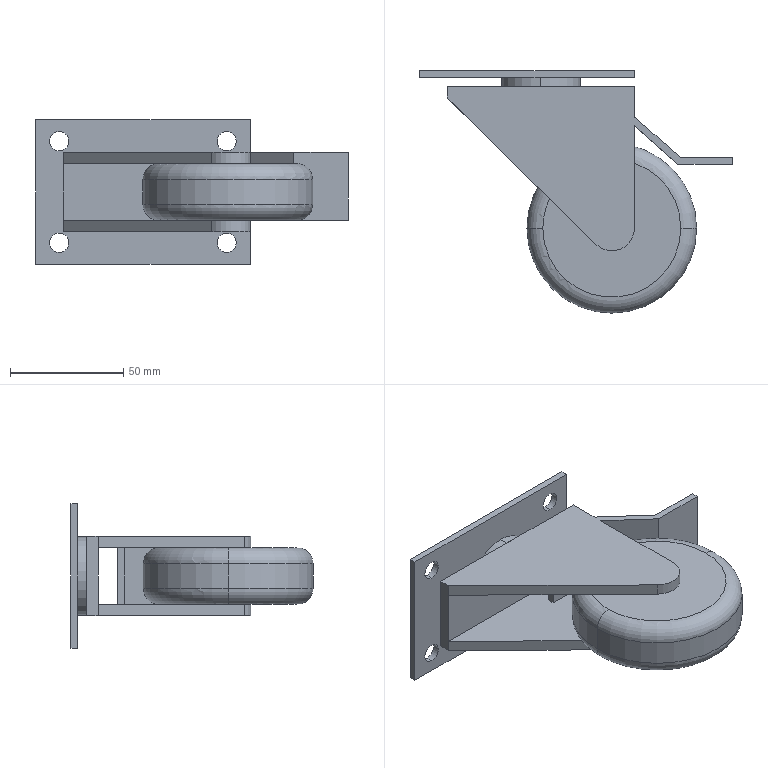Part | SolidWorks | features ICE 7, BossThin 1, Extrusion 1, Fillet 1, MirrorPattern 1 | 1 solid | 47 faces | box 138.347 x 107 x 64 mm | volume 180748 mm3 | plane 29 | cylinder 14 | torus 4 | commonest cylinder face diameters 8.5 x8 20 x2 35 x2 75 x2
STEP:
#1=CARTESIAN_POINT('',(-37.5,0.,5.5));
#2=VERTEX_POINT('',#1);
#3=CARTESIAN_POINT('',(37.5,0.,5.5));
#4=VERTEX_POINT('',#3);
#5=CARTESIAN_POINT('',(0.,0.,5.5));
#6=DIRECTION('',(0.,0.,-1.));
#7=DIRECTION('',(1.,0.,0.));
#8=AXIS2_PLACEMENT_3D('',#5,#6,#7);
#9=CIRCLE('',#8,37.5);
#10=EDGE_CURVE('',#2,#4,#9,.T.);
#11=ORIENTED_EDGE('',*,*,#10,.F.);
#12=CARTESIAN_POINT('',(-30.5,0.,12.5));
#13=VERTEX_POINT('',#12);
#14=CARTESIAN_POINT('',(-30.5,0.,5.5));
#15=DIRECTION('',(0.,1.,0.));
#16=DIRECTION('',(-1.,0.,0.));
#17=AXIS2_PLACEMENT_3D('',#14,#15,#16);
#18=CIRCLE('',#17,7.);
#19=EDGE_CURVE('',#2,#13,#18,.T.);
#20=ORIENTED_EDGE('',*,*,#19,.T.);
#21=CARTESIAN_POINT('',(-27.561,13.062,12.5));
#22=VERTEX_POINT('',#21);
#23=CARTESIAN_POINT('',(0.,0.,12.5));
#24=DIRECTION('',(0.,0.,1.));
#25=DIRECTION('',(1.,0.,0.));
#26=AXIS2_PLACEMENT_3D('',#23,#24,#25);
#27=CIRCLE('',#26,30.5);
#28=EDGE_CURVE('',#22,#13,#27,.T.);
#29=ORIENTED_EDGE('',*,*,#28,.F.);
#30=CARTESIAN_POINT('',(10.,28.814,12.5));
#31=VERTEX_POINT('',#30);
#32=CARTESIAN_POINT('',(0.,0.,12.5));
#33=DIRECTION('',(0.,0.,1.));
#34=DIRECTION('',(1.,0.,0.));
#35=AXIS2_PLACEMENT_3D('',#32,#33,#34);
#36=CIRCLE('',#35,30.5);
#37=EDGE_CURVE('',#31,#22,#36,.T.);
#38=ORIENTED_EDGE('',*,*,#37,.F.);
#39=CARTESIAN_POINT('',(30.5,0.,12.5));
#40=VERTEX_POINT('',#39);
#41=CARTESIAN_POINT('',(0.,0.,12.5));
#42=DIRECTION('',(0.,0.,1.));
#43=DIRECTION('',(1.,0.,0.));
#44=AXIS2_PLACEMENT_3D('',#41,#42,#43);
#45=CIRCLE('',#44,30.5);
#46=EDGE_CURVE('',#40,#31,#45,.T.);
#47=ORIENTED_EDGE('',*,*,#46,.F.);
#48=CARTESIAN_POINT('',(30.5,0.,5.5));
#49=DIRECTION('',(0.,-1.,0.));
#50=DIRECTION('',(0.,0.,-1.));
#51=AXIS2_PLACEMENT_3D('',#48,#49,#50);
#52=CIRCLE('',#51,7.);
#53=EDGE_CURVE('',#4,#40,#52,.T.);
#54=ORIENTED_EDGE('',*,*,#53,.F.);
#55=EDGE_LOOP('',(#11,#20,#29,#38,#47,#54));
#56=FACE_OUTER_BOUND('',#55,.T.);
#57=CARTESIAN_POINT('',(0.,0.,5.5));
#58=DIRECTION('',(0.,0.,1.));
#59=DIRECTION('',(1.,0.,0.));
#60=AXIS2_PLACEMENT_3D('',#57,#58,#59);
#61=TOROIDAL_SURFACE('',#60,30.5,7.);
#62=ADVANCED_FACE('',(#56),#61,.T.);
#63=CARTESIAN_POINT('',(-30.5,0.,-12.5));
#64=VERTEX_POINT('',#63);
#65=CARTESIAN_POINT('',(-27.561,13.062,-12.5));
#66=VERTEX_POINT('',#65);
#67=CARTESIAN_POINT('',(0.,0.,-12.5));
#68=DIRECTION('',(0.,0.,-1.));
#69=DIRECTION('',(1.,0.,0.));
#70=AXIS2_PLACEMENT_3D('',#67,#68,#69);
#71=CIRCLE('',#70,30.5);
#72=EDGE_CURVE('',#64,#66,#71,.T.);
#73=ORIENTED_EDGE('',*,*,#72,.F.);
#74=CARTESIAN_POINT('',(-37.5,0.,-5.5));
#75=VERTEX_POINT('',#74);
#76=CARTESIAN_POINT('',(-30.5,0.,-5.5));
#77=DIRECTION('',(0.,1.,0.));
#78=DIRECTION('',(-1.,0.,0.));
#79=AXIS2_PLACEMENT_3D('',#76,#77,#78);
#80=CIRCLE('',#79,7.);
#81=EDGE_CURVE('',#64,#75,#80,.T.);
#82=ORIENTED_EDGE('',*,*,#81,.T.);
#83=CARTESIAN_POINT('',(37.5,0.,-5.5));
#84=VERTEX_POINT('',#83);
#85=CARTESIAN_POINT('',(0.,0.,-5.5));
#86=DIRECTION('',(0.,0.,1.));
#87=DIRECTION('',(1.,0.,0.));
#88=AXIS2_PLACEMENT_3D('',#85,#86,#87);
#89=CIRCLE('',#88,37.5);
#90=EDGE_CURVE('',#84,#75,#89,.T.);
#91=ORIENTED_EDGE('',*,*,#90,.F.);
#92=CARTESIAN_POINT('',(30.5,0.,-12.5));
#93=VERTEX_POINT('',#92);
#94=CARTESIAN_POINT('',(30.5,0.,-5.5));
#95=DIRECTION('',(0.,-1.,0.));
#96=DIRECTION('',(0.,0.,-1.));
#97=AXIS2_PLACEMENT_3D('',#94,#95,#96);
#98=CIRCLE('',#97,7.);
#99=EDGE_CURVE('',#93,#84,#98,.T.);
#100=ORIENTED_EDGE('',*,*,#99,.F.);
#101=CARTESIAN_POINT('',(10.,28.814,-12.5));
#102=VERTEX_POINT('',#101);
#103=CARTESIAN_POINT('',(0.,0.,-12.5));
#104=DIRECTION('',(0.,0.,-1.));
#105=DIRECTION('',(1.,0.,0.));
#106=AXIS2_PLACEMENT_3D('',#103,#104,#105);
#107=CIRCLE('',#106,30.5);
#108=EDGE_CURVE('',#102,#93,#107,.T.);
#109=ORIENTED_EDGE('',*,*,#108,.F.);
#110=CARTESIAN_POINT('',(0.,0.,-12.5));
#111=DIRECTION('',(0.,0.,-1.));
#112=DIRECTION('',(1.,0.,0.));
#113=AXIS2_PLACEMENT_3D('',#110,#111,#112);
#114=CIRCLE('',#113,30.5);
#115=EDGE_CURVE('',#66,#102,#114,.T.);
#116=ORIENTED_EDGE('',*,*,#115,.F.);
#117=EDGE_LOOP('',(#73,#82,#91,#100,#109,#116));
#118=FACE_OUTER_BOUND('',#117,.T.);
#119=CARTESIAN_POINT('',(0.,0.,-5.5));
#120=DIRECTION('',(0.,0.,1.));
#121=DIRECTION('',(1.,0.,0.));
#122=AXIS2_PLACEMENT_3D('',#119,#120,#121);
#123=TOROIDAL_SURFACE('',#122,30.5,7.);
#124=ADVANCED_FACE('',(#118),#123,.T.);
#125=ORIENTED_EDGE('',*,*,#10,.T.);
#126=CARTESIAN_POINT('',(37.5,0.,12.5));
#127=DIRECTION('',(0.,0.,-1.));
#128=VECTOR('',#127,1000.);
#129=LINE('',#126,#128);
#130=EDGE_CURVE('',#4,#84,#129,.T.);
#131=ORIENTED_EDGE('',*,*,#130,.T.);
#132=ORIENTED_EDGE('',*,*,#90,.T.);
#133=CARTESIAN_POINT('',(-37.5,0.,12.5));
#134=DIRECTION('',(0.,0.,-1.));
#135=VECTOR('',#134,1000.);
#136=LINE('',#133,#135);
#137=EDGE_CURVE('',#2,#75,#136,.T.);
#138=ORIENTED_EDGE('',*,*,#137,.F.);
#139=EDGE_LOOP('',(#125,#131,#132,#138));
#140=FACE_OUTER_BOUND('',#139,.T.);
#141=CARTESIAN_POINT('',(0.,0.,12.5));
#142=DIRECTION('',(0.,0.,-1.));
#143=DIRECTION('',(-1.,0.,0.));
#144=AXIS2_PLACEMENT_3D('',#141,#142,#143);
#145=CYLINDRICAL_SURFACE('',#144,37.5);
#146=ADVANCED_FACE('',(#140),#145,.T.);
#147=CARTESIAN_POINT('',(-31.403,66.5,-17.5));
#148=VERTEX_POINT('',#147);
#149=CARTESIAN_POINT('',(-31.403,66.5,17.5));
#150=VERTEX_POINT('',#149);
#151=CARTESIAN_POINT('',(-31.403,66.5,0.));
#152=DIRECTION('',(0.,-1.,0.));
#153=DIRECTION('',(0.,0.,1.));
#154=AXIS2_PLACEMENT_3D('',#151,#152,#153);
#155=CIRCLE('',#154,17.5);
#156=EDGE_CURVE('',#148,#150,#155,.T.);
#157=ORIENTED_EDGE('',*,*,#156,.T.);
#158=CARTESIAN_POINT('',(-31.403,62.518,17.5));
#159=VERTEX_POINT('',#158);
#160=CARTESIAN_POINT('',(-31.403,115.997,17.5));
#161=DIRECTION('',(0.,-1.,0.));
#162=VECTOR('',#161,1000.);
#163=LINE('',#160,#162);
#164=EDGE_CURVE('',#150,#159,#163,.T.);
#165=ORIENTED_EDGE('',*,*,#164,.T.);
#166=CARTESIAN_POINT('',(-31.403,62.518,-17.5));
#167=VERTEX_POINT('',#166);
#168=CARTESIAN_POINT('',(-31.403,62.518,0.));
#169=DIRECTION('',(0.,1.,0.));
#170=DIRECTION('',(0.,0.,1.));
#171=AXIS2_PLACEMENT_3D('',#168,#169,#170);
#172=CIRCLE('',#171,17.5);
#173=EDGE_CURVE('',#159,#167,#172,.T.);
#174=ORIENTED_EDGE('',*,*,#173,.T.);
#175=CARTESIAN_POINT('',(-31.403,115.997,-17.5));
#176=DIRECTION('',(0.,-1.,0.));
#177=VECTOR('',#176,1000.);
#178=LINE('',#175,#177);
#179=EDGE_CURVE('',#148,#167,#178,.T.);
#180=ORIENTED_EDGE('',*,*,#179,.F.);
#181=EDGE_LOOP('',(#157,#165,#174,#180));
#182=FACE_OUTER_BOUND('',#181,.T.);
#183=CARTESIAN_POINT('',(-31.403,115.997,0.));
#184=DIRECTION('',(0.,-1.,0.));
#185=DIRECTION('',(0.,0.,-1.));
#186=AXIS2_PLACEMENT_3D('',#183,#184,#185);
#187=CYLINDRICAL_SURFACE('',#186,17.5);
#188=ADVANCED_FACE('',(#182),#187,.T.);
#189=CARTESIAN_POINT('',(-74.5,66.5,18.15));
#190=VERTEX_POINT('',#189);
#191=CARTESIAN_POINT('',(-74.5,66.5,26.65));
#192=VERTEX_POINT('',#191);
#193=CARTESIAN_POINT('',(-74.5,66.5,22.4));
#194=DIRECTION('',(0.,1.,0.));
#195=DIRECTION('',(0.,0.,1.));
#196=AXIS2_PLACEMENT_3D('',#193,#194,#195);
#197=CIRCLE('',#196,4.25);
#198=EDGE_CURVE('',#190,#192,#197,.T.);
#199=ORIENTED_EDGE('',*,*,#198,.F.);
#200=CARTESIAN_POINT('',(-74.5,69.5,18.15));
#201=VERTEX_POINT('',#200);
#202=CARTESIAN_POINT('',(-74.5,-37.5,18.15));
#203=DIRECTION('',(0.,1.,0.));
#204=VECTOR('',#203,1000.);
#205=LINE('',#202,#204);
#206=EDGE_CURVE('',#190,#201,#205,.T.);
#207=ORIENTED_EDGE('',*,*,#206,.T.);
#208=CARTESIAN_POINT('',(-74.5,69.5,26.65));
#209=VERTEX_POINT('',#208);
#210=CARTESIAN_POINT('',(-74.5,69.5,22.4));
#211=DIRECTION('',(0.,1.,0.));
#212=DIRECTION('',(0.,0.,1.));
#213=AXIS2_PLACEMENT_3D('',#210,#211,#212);
#214=CIRCLE('',#213,4.25);
#215=EDGE_CURVE('',#201,#209,#214,.T.);
#216=ORIENTED_EDGE('',*,*,#215,.T.);
#217=CARTESIAN_POINT('',(-74.5,-37.5,26.65));
#218=DIRECTION('',(0.,1.,0.));
#219=VECTOR('',#218,1000.);
#220=LINE('',#217,#219);
#221=EDGE_CURVE('',#192,#209,#220,.T.);
#222=ORIENTED_EDGE('',*,*,#221,.F.);
#223=EDGE_LOOP('',(#199,#207,#216,#222));
#224=FACE_OUTER_BOUND('',#223,.T.);
#225=CARTESIAN_POINT('',(-74.5,-37.5,22.4));
#226=DIRECTION('',(0.,1.,0.));
#227=DIRECTION('',(0.,0.,1.));
#228=AXIS2_PLACEMENT_3D('',#225,#226,#227);
#229=CYLINDRICAL_SURFACE('',#228,4.25);
#230=ADVANCED_FACE('',(#224),#229,.F.);
#231=CARTESIAN_POINT('',(-0.5,66.5,18.15));
#232=VERTEX_POINT('',#231);
#233=CARTESIAN_POINT('',(-0.5,66.5,26.65));
#234=VERTEX_POINT('',#233);
#235=CARTESIAN_POINT('',(-0.5,66.5,22.4));
#236=DIRECTION('',(0.,1.,0.));
#237=DIRECTION('',(0.,0.,1.));
#238=AXIS2_PLACEMENT_3D('',#235,#236,#237);
#239=CIRCLE('',#238,4.25);
#240=EDGE_CURVE('',#232,#234,#239,.T.);
#241=ORIENTED_EDGE('',*,*,#240,.F.);
#242=CARTESIAN_POINT('',(-0.5,69.5,18.15));
#243=VERTEX_POINT('',#242);
#244=CARTESIAN_POINT('',(-0.5,-37.5,18.15));
#245=DIRECTION('',(0.,1.,0.));
#246=VECTOR('',#245,1000.);
#247=LINE('',#244,#246);
#248=EDGE_CURVE('',#232,#243,#247,.T.);
#249=ORIENTED_EDGE('',*,*,#248,.T.);
#250=CARTESIAN_POINT('',(-0.5,69.5,26.65));
#251=VERTEX_POINT('',#250);
#252=CARTESIAN_POINT('',(-0.5,69.5,22.4));
#253=DIRECTION('',(0.,1.,0.));
#254=DIRECTION('',(0.,0.,1.));
#255=AXIS2_PLACEMENT_3D('',#252,#253,#254);
#256=CIRCLE('',#255,4.25);
#257=EDGE_CURVE('',#243,#251,#256,.T.);
#258=ORIENTED_EDGE('',*,*,#257,.T.);
#259=CARTESIAN_POINT('',(-0.5,-37.5,26.65));
#260=DIRECTION('',(0.,1.,0.));
#261=VECTOR('',#260,1000.);
#262=LINE('',#259,#261);
#263=EDGE_CURVE('',#234,#251,#262,.T.);
#264=ORIENTED_EDGE('',*,*,#263,.F.);
#265=EDGE_LOOP('',(#241,#249,#258,#264));
#266=FACE_OUTER_BOUND('',#265,.T.);
#267=CARTESIAN_POINT('',(-0.5,-37.5,22.4));
#268=DIRECTION('',(0.,1.,0.));
#269=DIRECTION('',(0.,0.,1.));
#270=AXIS2_PLACEMENT_3D('',#267,#268,#269);
#271=CYLINDRICAL_SURFACE('',#270,4.25);
#272=ADVANCED_FACE('',(#266),#271,.F.);
#273=CARTESIAN_POINT('',(-0.5,66.5,-26.65));
#274=VERTEX_POINT('',#273);
#275=CARTESIAN_POINT('',(-0.5,66.5,-18.15));
#276=VERTEX_POINT('',#275);
#277=CARTESIAN_POINT('',(-0.5,66.5,-22.4));
#278=DIRECTION('',(0.,1.,0.));
#279=DIRECTION('',(0.,0.,1.));
#280=AXIS2_PLACEMENT_3D('',#277,#278,#279);
#281=CIRCLE('',#280,4.25);
#282=EDGE_CURVE('',#274,#276,#281,.T.);
#283=ORIENTED_EDGE('',*,*,#282,.F.);
#284=CARTESIAN_POINT('',(-0.5,69.5,-26.65));
#285=VERTEX_POINT('',#284);
#286=CARTESIAN_POINT('',(-0.5,-37.5,-26.65));
#287=DIRECTION('',(0.,1.,0.));
#288=VECTOR('',#287,1000.);
#289=LINE('',#286,#288);
#290=EDGE_CURVE('',#274,#285,#289,.T.);
#291=ORIENTED_EDGE('',*,*,#290,.T.);
#292=CARTESIAN_POINT('',(-0.5,69.5,-18.15));
#293=VERTEX_POINT('',#292);
#294=CARTESIAN_POINT('',(-0.5,69.5,-22.4));
#295=DIRECTION('',(0.,1.,0.));
#296=DIRECTION('',(0.,0.,1.));
#297=AXIS2_PLACEMENT_3D('',#294,#295,#296);
#298=CIRCLE('',#297,4.25);
#299=EDGE_CURVE('',#285,#293,#298,.T.);
#300=ORIENTED_EDGE('',*,*,#299,.T.);
#301=CARTESIAN_POINT('',(-0.5,-37.5,-18.15));
#302=DIRECTION('',(0.,1.,0.));
#303=VECTOR('',#302,1000.);
#304=LINE('',#301,#303);
#305=EDGE_CURVE('',#276,#293,#304,.T.);
#306=ORIENTED_EDGE('',*,*,#305,.F.);
#307=EDGE_LOOP('',(#283,#291,#300,#306));
#308=FACE_OUTER_BOUND('',#307,.T.);
#309=CARTESIAN_POINT('',(-0.5,-37.5,-22.4));
#310=DIRECTION('',(0.,1.,0.));
#311=DIRECTION('',(0.,0.,1.));
#312=AXIS2_PLACEMENT_3D('',#309,#310,#311);
#313=CYLINDRICAL_SURFACE('',#312,4.25);
#314=ADVANCED_FACE('',(#308),#313,.F.);
#315=CARTESIAN_POINT('',(-74.5,66.5,-26.65));
#316=VERTEX_POINT('',#315);
#317=CARTESIAN_POINT('',(-74.5,66.5,-18.15));
#318=VERTEX_POINT('',#317);
#319=CARTESIAN_POINT('',(-74.5,66.5,-22.4));
#320=DIRECTION('',(0.,1.,0.));
#321=DIRECTION('',(0.,0.,1.));
#322=AXIS2_PLACEMENT_3D('',#319,#320,#321);
#323=CIRCLE('',#322,4.25);
#324=EDGE_CURVE('',#316,#318,#323,.T.);
#325=ORIENTED_EDGE('',*,*,#324,.F.);
#326=CARTESIAN_POINT('',(-74.5,69.5,-26.65));
#327=VERTEX_POINT('',#326);
#328=CARTESIAN_POINT('',(-74.5,-37.5,-26.65));
#329=DIRECTION('',(0.,1.,0.));
#330=VECTOR('',#329,1000.);
#331=LINE('',#328,#330);
#332=EDGE_CURVE('',#316,#327,#331,.T.);
#333=ORIENTED_EDGE('',*,*,#332,.T.);
#334=CARTESIAN_POINT('',(-74.5,69.5,-18.15));
#335=VERTEX_POINT('',#334);
#336=CARTESIAN_POINT('',(-74.5,69.5,-22.4));
#337=DIRECTION('',(0.,1.,0.));
#338=DIRECTION('',(0.,0.,1.));
#339=AXIS2_PLACEMENT_3D('',#336,#337,#338);
#340=CIRCLE('',#339,4.25);
#341=EDGE_CURVE('',#327,#335,#340,.T.);
#342=ORIENTED_EDGE('',*,*,#341,.T.);
#343=CARTESIAN_POINT('',(-74.5,-37.5,-18.15));
#344=DIRECTION('',(0.,1.,0.));
#345=VECTOR('',#344,1000.);
#346=LINE('',#343,#345);
#347=EDGE_CURVE('',#318,#335,#346,.T.);
#348=ORIENTED_EDGE('',*,*,#347,.F.);
#349=EDGE_LOOP('',(#325,#333,#342,#348));
#350=FACE_OUTER_BOUND('',#349,.T.);
#351=CARTESIAN_POINT('',(-74.5,-37.5,-22.4));
#352=DIRECTION('',(0.,1.,0.));
#353=DIRECTION('',(0.,0.,1.));
#354=AXIS2_PLACEMENT_3D('',#351,#352,#353);
#355=CYLINDRICAL_SURFACE('',#354,4.25);
#356=ADVANCED_FACE('',(#350),#355,.F.);
#357=CARTESIAN_POINT('',(10.,48.792,12.5));
#358=VERTEX_POINT('',#357);
#359=CARTESIAN_POINT('',(10.,48.792,17.5));
#360=VERTEX_POINT('',#359);
#361=CARTESIAN_POINT('',(10.,48.792,17.5));
#362=DIRECTION('',(0.,0.,1.));
#363=VECTOR('',#362,1000.);
#364=LINE('',#361,#363);
#365=EDGE_CURVE('',#358,#360,#364,.T.);
#366=ORIENTED_EDGE('',*,*,#365,.F.);
#367=CARTESIAN_POINT('',(10.,57.518,12.5));
#368=VERTEX_POINT('',#367);
#369=CARTESIAN_POINT('',(10.,69.5,12.5));
#370=DIRECTION('',(0.,1.,0.));
#371=VECTOR('',#370,1000.);
#372=LINE('',#369,#371);
#373=EDGE_CURVE('',#358,#368,#372,.T.);
#374=ORIENTED_EDGE('',*,*,#373,.T.);
#375=CARTESIAN_POINT('',(10.,57.518,-12.5));
#376=VERTEX_POINT('',#375);
#377=CARTESIAN_POINT('',(10.,57.518,-17.5));
#378=DIRECTION('',(0.,0.,-1.));
#379=VECTOR('',#378,1000.);
#380=LINE('',#377,#379);
#381=EDGE_CURVE('',#368,#376,#380,.T.);
#382=ORIENTED_EDGE('',*,*,#381,.T.);
#383=CARTESIAN_POINT('',(10.,48.792,-12.5));
#384=VERTEX_POINT('',#383);
#385=CARTESIAN_POINT('',(10.,69.5,-12.5));
#386=DIRECTION('',(0.,1.,0.));
#387=VECTOR('',#386,1000.);
#388=LINE('',#385,#387);
#389=EDGE_CURVE('',#384,#376,#388,.T.);
#390=ORIENTED_EDGE('',*,*,#389,.F.);
#391=CARTESIAN_POINT('',(10.,45.286,-12.5));
#392=VERTEX_POINT('',#391);
#393=CARTESIAN_POINT('',(10.,69.5,-12.5));
#394=DIRECTION('',(0.,1.,0.));
#395=VECTOR('',#394,1000.);
#396=LINE('',#393,#395);
#397=EDGE_CURVE('',#392,#384,#396,.T.);
#398=ORIENTED_EDGE('',*,*,#397,.F.);
#399=CARTESIAN_POINT('',(10.,69.5,-12.5));
#400=DIRECTION('',(0.,1.,0.));
#401=VECTOR('',#400,1000.);
#402=LINE('',#399,#401);
#403=EDGE_CURVE('',#102,#392,#402,.T.);
#404=ORIENTED_EDGE('',*,*,#403,.F.);
#405=CARTESIAN_POINT('',(10.,0.,-12.5));
#406=VERTEX_POINT('',#405);
#407=CARTESIAN_POINT('',(10.,69.5,-12.5));
#408=DIRECTION('',(0.,1.,0.));
#409=VECTOR('',#408,1000.);
#410=LINE('',#407,#409);
#411=EDGE_CURVE('',#406,#102,#410,.T.);
#412=ORIENTED_EDGE('',*,*,#411,.F.);
#413=CARTESIAN_POINT('',(10.,0.,-17.5));
#414=VERTEX_POINT('',#413);
#415=CARTESIAN_POINT('',(10.,0.,-17.5));
#416=DIRECTION('',(0.,0.,1.));
#417=VECTOR('',#416,1000.);
#418=LINE('',#415,#417);
#419=EDGE_CURVE('',#414,#406,#418,.T.);
#420=ORIENTED_EDGE('',*,*,#419,.F.);
#421=CARTESIAN_POINT('',(10.,62.518,-17.5));
#422=VERTEX_POINT('',#421);
#423=CARTESIAN_POINT('',(10.,69.5,-17.5));
#424=DIRECTION('',(0.,1.,0.));
#425=VECTOR('',#424,1000.);
#426=LINE('',#423,#425);
#427=EDGE_CURVE('',#414,#422,#426,.T.);
#428=ORIENTED_EDGE('',*,*,#427,.T.);
#429=CARTESIAN_POINT('',(10.,62.518,17.5));
#430=VERTEX_POINT('',#429);
#431=CARTESIAN_POINT('',(10.,62.518,-17.5));
#432=DIRECTION('',(0.,0.,-1.));
#433=VECTOR('',#432,1000.);
#434=LINE('',#431,#433);
#435=EDGE_CURVE('',#430,#422,#434,.T.);
#436=ORIENTED_EDGE('',*,*,#435,.F.);
#437=CARTESIAN_POINT('',(10.,69.5,17.5));
#438=DIRECTION('',(0.,1.,0.));
#439=VECTOR('',#438,1000.);
#440=LINE('',#437,#439);
#441=EDGE_CURVE('',#360,#430,#440,.T.);
#442=ORIENTED_EDGE('',*,*,#441,.F.);
#443=EDGE_LOOP('',(#366,#374,#382,#390,#398,#404,#412,#420,#428,#436,#442));
#444=FACE_OUTER_BOUND('',#443,.T.);
#445=CARTESIAN_POINT('',(10.,69.5,17.5));
#446=DIRECTION('',(-1.,0.,0.));
#447=DIRECTION('',(0.,-1.,0.));
#448=AXIS2_PLACEMENT_3D('',#445,#446,#447);
#449=PLANE('',#448);
#450=ADVANCED_FACE('',(#444),#449,.F.);
#451=CARTESIAN_POINT('',(-74.5,66.5,-22.4));
#452=DIRECTION('',(0.,1.,0.));
#453=DIRECTION('',(0.,0.,1.));
#454=AXIS2_PLACEMENT_3D('',#451,#452,#453);
#455=CIRCLE('',#454,4.25);
#456=EDGE_CURVE('',#318,#316,#455,.T.);
#457=ORIENTED_EDGE('',*,*,#456,.T.);
#458=ORIENTED_EDGE('',*,*,#324,.T.);
#459=EDGE_LOOP('',(#457,#458));
#460=FACE_BOUND('',#459,.T.);
#461=CARTESIAN_POINT('',(-0.5,66.5,-22.4));
#462=DIRECTION('',(0.,1.,0.));
#463=DIRECTION('',(0.,0.,1.));
#464=AXIS2_PLACEMENT_3D('',#461,#462,#463);
#465=CIRCLE('',#464,4.25);
#466=EDGE_CURVE('',#276,#274,#465,.T.);
#467=ORIENTED_EDGE('',*,*,#466,.T.);
#468=ORIENTED_EDGE('',*,*,#282,.T.);
#469=EDGE_LOOP('',(#467,#468));
#470=FACE_BOUND('',#469,.T.);
#471=CARTESIAN_POINT('',(-0.5,66.5,22.4));
#472=DIRECTION('',(0.,1.,0.));
#473=DIRECTION('',(0.,0.,1.));
#474=AXIS2_PLACEMENT_3D('',#471,#472,#473);
#475=CIRCLE('',#474,4.25);
#476=EDGE_CURVE('',#234,#232,#475,.T.);
#477=ORIENTED_EDGE('',*,*,#476,.T.);
#478=ORIENTED_EDGE('',*,*,#240,.T.);
#479=EDGE_LOOP('',(#477,#478));
#480=FACE_BOUND('',#479,.T.);
#481=CARTESIAN_POINT('',(-74.5,66.5,22.4));
#482=DIRECTION('',(0.,1.,0.));
#483=DIRECTION('',(0.,0.,1.));
#484=AXIS2_PLACEMENT_3D('',#481,#482,#483);
#485=CIRCLE('',#484,4.25);
#486=EDGE_CURVE('',#192,#190,#485,.T.);
#487=ORIENTED_EDGE('',*,*,#486,.T.);
#488=ORIENTED_EDGE('',*,*,#198,.T.);
#489=EDGE_LOOP('',(#487,#488));
#490=FACE_BOUND('',#489,.T.);
#491=CARTESIAN_POINT('',(10.,66.5,-32.));
#492=VERTEX_POINT('',#491);
#493=CARTESIAN_POINT('',(-85.,66.5,-32.));
#494=VERTEX_POINT('',#493);
#495=CARTESIAN_POINT('',(-85.,66.5,-32.));
#496=DIRECTION('',(-1.,0.,0.));
#497=VECTOR('',#496,1000.);
#498=LINE('',#495,#497);
#499=EDGE_CURVE('',#492,#494,#498,.T.);
#500=ORIENTED_EDGE('',*,*,#499,.F.);
#501=CARTESIAN_POINT('',(10.,66.5,32.));
#502=VERTEX_POINT('',#501);
#503=CARTESIAN_POINT('',(10.,66.5,-32.));
#504=DIRECTION('',(0.,0.,-1.));
#505=VECTOR('',#504,1000.);
#506=LINE('',#503,#505);
#507=EDGE_CURVE('',#502,#492,#506,.T.);
#508=ORIENTED_EDGE('',*,*,#507,.F.);
#509=CARTESIAN_POINT('',(-85.,66.5,32.));
#510=VERTEX_POINT('',#509);
#511=CARTESIAN_POINT('',(-85.,66.5,32.));
#512=DIRECTION('',(1.,0.,0.));
#513=VECTOR('',#512,1000.);
#514=LINE('',#511,#513);
#515=EDGE_CURVE('',#510,#502,#514,.T.);
#516=ORIENTED_EDGE('',*,*,#515,.F.);
#517=CARTESIAN_POINT('',(-85.,66.5,-32.));
#518=DIRECTION('',(0.,0.,1.));
#519=VECTOR('',#518,1000.);
#520=LINE('',#517,#519);
#521=EDGE_CURVE('',#494,#510,#520,.T.);
#522=ORIENTED_EDGE('',*,*,#521,.F.);
#523=EDGE_LOOP('',(#500,#508,#516,#522));
#524=FACE_OUTER_BOUND('',#523,.T.);
#525=ORIENTED_EDGE('',*,*,#156,.F.);
#526=CARTESIAN_POINT('',(-31.403,66.5,0.));
#527=DIRECTION('',(0.,-1.,0.));
#528=DIRECTION('',(0.,0.,1.));
#529=AXIS2_PLACEMENT_3D('',#526,#527,#528);
#530=CIRCLE('',#529,17.5);
#531=EDGE_CURVE('',#150,#148,#530,.T.);
#532=ORIENTED_EDGE('',*,*,#531,.F.);
#533=EDGE_LOOP('',(#525,#532));
#534=FACE_BOUND('',#533,.T.);
#535=CARTESIAN_POINT('',(-85.,66.5,32.));
#536=DIRECTION('',(0.,1.,0.));
#537=DIRECTION('',(0.,0.,1.));
#538=AXIS2_PLACEMENT_3D('',#535,#536,#537);
#539=PLANE('',#538);
#540=ADVANCED_FACE('',(#460,#470,#480,#490,#524,#534),#539,.F.);
#541=ORIENTED_EDGE('',*,*,#332,.F.);
#542=ORIENTED_EDGE('',*,*,#456,.F.);
#543=ORIENTED_EDGE('',*,*,#347,.T.);
#544=CARTESIAN_POINT('',(-74.5,69.5,-22.4));
#545=DIRECTION('',(0.,1.,0.));
#546=DIRECTION('',(0.,0.,1.));
#547=AXIS2_PLACEMENT_3D('',#544,#545,#546);
#548=CIRCLE('',#547,4.25);
#549=EDGE_CURVE('',#335,#327,#548,.T.);
#550=ORIENTED_EDGE('',*,*,#549,.T.);
#551=EDGE_LOOP('',(#541,#542,#543,#550));
#552=FACE_OUTER_BOUND('',#551,.T.);
#553=CARTESIAN_POINT('',(-74.5,-37.5,-22.4));
#554=DIRECTION('',(0.,1.,0.));
#555=DIRECTION('',(0.,0.,1.));
#556=AXIS2_PLACEMENT_3D('',#553,#554,#555);
#557=CYLINDRICAL_SURFACE('',#556,4.25);
#558=ADVANCED_FACE('',(#552),#557,.F.);
#559=ORIENTED_EDGE('',*,*,#290,.F.);
#560=ORIENTED_EDGE('',*,*,#466,.F.);
#561=ORIENTED_EDGE('',*,*,#305,.T.);
#562=CARTESIAN_POINT('',(-0.5,69.5,-22.4));
#563=DIRECTION('',(0.,1.,0.));
#564=DIRECTION('',(0.,0.,1.));
#565=AXIS2_PLACEMENT_3D('',#562,#563,#564);
#566=CIRCLE('',#565,4.25);
#567=EDGE_CURVE('',#293,#285,#566,.T.);
#568=ORIENTED_EDGE('',*,*,#567,.T.);
#569=EDGE_LOOP('',(#559,#560,#561,#568));
#570=FACE_OUTER_BOUND('',#569,.T.);
#571=CARTESIAN_POINT('',(-0.5,-37.5,-22.4));
#572=DIRECTION('',(0.,1.,0.));
#573=DIRECTION('',(0.,0.,1.));
#574=AXIS2_PLACEMENT_3D('',#571,#572,#573);
#575=CYLINDRICAL_SURFACE('',#574,4.25);
#576=ADVANCED_FACE('',(#570),#575,.F.);
#577=CARTESIAN_POINT('',(-74.5,69.5,22.4));
#578=DIRECTION('',(0.,1.,0.));
#579=DIRECTION('',(0.,0.,1.));
#580=AXIS2_PLACEMENT_3D('',#577,#578,#579);
#581=CIRCLE('',#580,4.25);
#582=EDGE_CURVE('',#209,#201,#581,.T.);
#583=ORIENTED_EDGE('',*,*,#582,.F.);
#584=ORIENTED_EDGE('',*,*,#215,.F.);
#585=EDGE_LOOP('',(#583,#584));
#586=FACE_BOUND('',#585,.T.);
#587=ORIENTED_EDGE('',*,*,#549,.F.);
#588=ORIENTED_EDGE('',*,*,#341,.F.);
#589=EDGE_LOOP('',(#587,#588));
#590=FACE_BOUND('',#589,.T.);
#591=ORIENTED_EDGE('',*,*,#567,.F.);
#592=ORIENTED_EDGE('',*,*,#299,.F.);
#593=EDGE_LOOP('',(#591,#592));
#594=FACE_BOUND('',#593,.T.);
#595=CARTESIAN_POINT('',(-0.5,69.5,22.4));
#596=DIRECTION('',(0.,1.,0.));
#597=DIRECTION('',(0.,0.,1.));
#598=AXIS2_PLACEMENT_3D('',#595,#596,#597);
#599=CIRCLE('',#598,4.25);
#600=EDGE_CURVE('',#251,#243,#599,.T.);
#601=ORIENTED_EDGE('',*,*,#600,.F.);
#602=ORIENTED_EDGE('',*,*,#257,.F.);
#603=EDGE_LOOP('',(#601,#602));
#604=FACE_BOUND('',#603,.T.);
#605=CARTESIAN_POINT('',(10.,69.5,32.));
#606=VERTEX_POINT('',#605);
#607=CARTESIAN_POINT('',(10.,69.5,-32.));
#608=VERTEX_POINT('',#607);
#609=CARTESIAN_POINT('',(10.,69.5,17.5));
#610=DIRECTION('',(0.,0.,-1.));
#611=VECTOR('',#610,1000.);
#612=LINE('',#609,#611);
#613=EDGE_CURVE('',#606,#608,#612,.T.);
#614=ORIENTED_EDGE('',*,*,#613,.T.);
#615=CARTESIAN_POINT('',(-85.,69.5,-32.));
#616=VERTEX_POINT('',#615);
#617=CARTESIAN_POINT('',(-85.,69.5,-32.));
#618=DIRECTION('',(-1.,0.,0.));
#619=VECTOR('',#618,1000.);
#620=LINE('',#617,#619);
#621=EDGE_CURVE('',#608,#616,#620,.T.);
#622=ORIENTED_EDGE('',*,*,#621,.T.);
#623=CARTESIAN_POINT('',(-85.,69.5,32.));
#624=VERTEX_POINT('',#623);
#625=CARTESIAN_POINT('',(-85.,69.5,17.5));
#626=DIRECTION('',(0.,0.,-1.));
#627=VECTOR('',#626,1000.);
#628=LINE('',#625,#627);
#629=EDGE_CURVE('',#624,#616,#628,.T.);
#630=ORIENTED_EDGE('',*,*,#629,.F.);
#631=CARTESIAN_POINT('',(-85.,69.5,32.));
#632=DIRECTION('',(1.,0.,0.));
#633=VECTOR('',#632,1000.);
#634=LINE('',#631,#633);
#635=EDGE_CURVE('',#624,#606,#634,.T.);
#636=ORIENTED_EDGE('',*,*,#635,.T.);
#637=EDGE_LOOP('',(#614,#622,#630,#636));
#638=FACE_OUTER_BOUND('',#637,.T.);
#639=CARTESIAN_POINT('',(-85.,69.5,17.5));
#640=DIRECTION('',(0.,-1.,0.));
#641=DIRECTION('',(0.,0.,-1.));
#642=AXIS2_PLACEMENT_3D('',#639,#640,#641);
#643=PLANE('',#642);
#644=ADVANCED_FACE('',(#586,#590,#594,#604,#638),#643,.F.);
#645=ORIENTED_EDGE('',*,*,#629,.T.);
#646=CARTESIAN_POINT('',(-85.,66.5,-32.));
#647=DIRECTION('',(0.,1.,0.));
#648=VECTOR('',#647,1000.);
#649=LINE('',#646,#648);
#650=EDGE_CURVE('',#494,#616,#649,.T.);
#651=ORIENTED_EDGE('',*,*,#650,.F.);
#652=ORIENTED_EDGE('',*,*,#521,.T.);
#653=CARTESIAN_POINT('',(-85.,66.5,32.));
#654=DIRECTION('',(0.,1.,0.));
#655=VECTOR('',#654,1000.);
#656=LINE('',#653,#655);
#657=EDGE_CURVE('',#510,#624,#656,.T.);
#658=ORIENTED_EDGE('',*,*,#657,.T.);
#659=EDGE_LOOP('',(#645,#651,#652,#658));
#660=FACE_OUTER_BOUND('',#659,.T.);
#661=CARTESIAN_POINT('',(-85.,66.5,-32.));
#662=DIRECTION('',(-1.,0.,0.));
#663=DIRECTION('',(0.,0.,1.));
#664=AXIS2_PLACEMENT_3D('',#661,#662,#663);
#665=PLANE('',#664);
#666=ADVANCED_FACE('',(#660),#665,.T.);
#667=ORIENTED_EDGE('',*,*,#635,.F.);
#668=ORIENTED_EDGE('',*,*,#657,.F.);
#669=ORIENTED_EDGE('',*,*,#515,.T.);
#670=CARTESIAN_POINT('',(10.,66.5,32.));
#671=DIRECTION('',(0.,1.,0.));
#672=VECTOR('',#671,1000.);
#673=LINE('',#670,#672);
#674=EDGE_CURVE('',#502,#606,#673,.T.);
#675=ORIENTED_EDGE('',*,*,#674,.T.);
#676=EDGE_LOOP('',(#667,#668,#669,#675));
#677=FACE_OUTER_BOUND('',#676,.T.);
#678=CARTESIAN_POINT('',(-85.,66.5,32.));
#679=DIRECTION('',(0.,0.,1.));
#680=DIRECTION('',(1.,0.,0.));
#681=AXIS2_PLACEMENT_3D('',#678,#679,#680);
#682=PLANE('',#681);
#683=ADVANCED_FACE('',(#677),#682,.T.);
#684=ORIENTED_EDGE('',*,*,#621,.F.);
#685=CARTESIAN_POINT('',(10.,66.5,-32.));
#686=DIRECTION('',(0.,1.,0.));
#687=VECTOR('',#686,1000.);
#688=LINE('',#685,#687);
#689=EDGE_CURVE('',#492,#608,#688,.T.);
#690=ORIENTED_EDGE('',*,*,#689,.F.);
#691=ORIENTED_EDGE('',*,*,#499,.T.);
#692=ORIENTED_EDGE('',*,*,#650,.T.);
#693=EDGE_LOOP('',(#684,#690,#691,#692));
#694=FACE_OUTER_BOUND('',#693,.T.);
#695=CARTESIAN_POINT('',(-85.,66.5,-32.));
#696=DIRECTION('',(0.,0.,-1.));
#697=DIRECTION('',(-1.,0.,0.));
#698=AXIS2_PLACEMENT_3D('',#695,#696,#697);
#699=PLANE('',#698);
#700=ADVANCED_FACE('',(#694),#699,.T.);
#701=ORIENTED_EDGE('',*,*,#248,.F.);
#702=ORIENTED_EDGE('',*,*,#476,.F.);
#703=ORIENTED_EDGE('',*,*,#263,.T.);
#704=ORIENTED_EDGE('',*,*,#600,.T.);
#705=EDGE_LOOP('',(#701,#702,#703,#704));
#706=FACE_OUTER_BOUND('',#705,.T.);
#707=CARTESIAN_POINT('',(-0.5,-37.5,22.4));
#708=DIRECTION('',(0.,1.,0.));
#709=DIRECTION('',(0.,0.,1.));
#710=AXIS2_PLACEMENT_3D('',#707,#708,#709);
#711=CYLINDRICAL_SURFACE('',#710,4.25);
#712=ADVANCED_FACE('',(#706),#711,.F.);
#713=ORIENTED_EDGE('',*,*,#206,.F.);
#714=ORIENTED_EDGE('',*,*,#486,.F.);
#715=ORIENTED_EDGE('',*,*,#221,.T.);
#716=ORIENTED_EDGE('',*,*,#582,.T.);
#717=EDGE_LOOP('',(#713,#714,#715,#716));
#718=FACE_OUTER_BOUND('',#717,.T.);
#719=CARTESIAN_POINT('',(-74.5,-37.5,22.4));
#720=DIRECTION('',(0.,1.,0.));
#721=DIRECTION('',(0.,0.,1.));
#722=AXIS2_PLACEMENT_3D('',#719,#720,#721);
#723=CYLINDRICAL_SURFACE('',#722,4.25);
#724=ADVANCED_FACE('',(#718),#723,.F.);
#725=ORIENTED_EDGE('',*,*,#674,.F.);
#726=ORIENTED_EDGE('',*,*,#507,.T.);
#727=ORIENTED_EDGE('',*,*,#689,.T.);
#728=ORIENTED_EDGE('',*,*,#613,.F.);
#729=EDGE_LOOP('',(#725,#726,#727,#728));
#730=FACE_OUTER_BOUND('',#729,.T.);
#731=CARTESIAN_POINT('',(10.,69.5,17.5));
#732=DIRECTION('',(-1.,0.,0.));
#733=DIRECTION('',(0.,-1.,0.));
#734=AXIS2_PLACEMENT_3D('',#731,#732,#733);
#735=PLANE('',#734);
#736=ADVANCED_FACE('',(#730),#735,.F.);
#737=ORIENTED_EDGE('',*,*,#164,.F.);
#738=ORIENTED_EDGE('',*,*,#531,.T.);
#739=ORIENTED_EDGE('',*,*,#179,.T.);
#740=CARTESIAN_POINT('',(-31.403,62.518,0.));
#741=DIRECTION('',(0.,1.,0.));
#742=DIRECTION('',(0.,0.,1.));
#743=AXIS2_PLACEMENT_3D('',#740,#741,#742);
#744=CIRCLE('',#743,17.5);
#745=EDGE_CURVE('',#167,#159,#744,.T.);
#746=ORIENTED_EDGE('',*,*,#745,.T.);
#747=EDGE_LOOP('',(#737,#738,#739,#746));
#748=FACE_OUTER_BOUND('',#747,.T.);
#749=CARTESIAN_POINT('',(-31.403,115.997,0.));
#750=DIRECTION('',(0.,-1.,0.));
#751=DIRECTION('',(0.,0.,-1.));
#752=AXIS2_PLACEMENT_3D('',#749,#750,#751);
#753=CYLINDRICAL_SURFACE('',#752,17.5);
#754=ADVANCED_FACE('',(#748),#753,.T.);
#755=ORIENTED_EDGE('',*,*,#173,.F.);
#756=CARTESIAN_POINT('',(10.,62.518,17.5));
#757=DIRECTION('',(1.,0.,0.));
#758=VECTOR('',#757,1000.);
#759=LINE('',#756,#758);
#760=EDGE_CURVE('',#159,#430,#759,.T.);
#761=ORIENTED_EDGE('',*,*,#760,.T.);
#762=ORIENTED_EDGE('',*,*,#435,.T.);
#763=CARTESIAN_POINT('',(10.,62.518,-17.5));
#764=DIRECTION('',(-1.,0.,0.));
#765=VECTOR('',#764,1000.);
#766=LINE('',#763,#765);
#767=EDGE_CURVE('',#422,#167,#766,.T.);
#768=ORIENTED_EDGE('',*,*,#767,.T.);
#769=EDGE_LOOP('',(#755,#761,#762,#768));
#770=FACE_OUTER_BOUND('',#769,.T.);
#771=CARTESIAN_POINT('',(0.,62.518,0.));
#772=DIRECTION('',(0.,-1.,0.));
#773=DIRECTION('',(0.,0.,-1.));
#774=AXIS2_PLACEMENT_3D('',#771,#772,#773);
#775=PLANE('',#774);
#776=ADVANCED_FACE('',(#770),#775,.F.);
#777=CARTESIAN_POINT('',(10.,45.286,12.5));
#778=VERTEX_POINT('',#777);
#779=CARTESIAN_POINT('',(10.,69.5,12.5));
#780=DIRECTION('',(0.,1.,0.));
#781=VECTOR('',#780,1000.);
#782=LINE('',#779,#781);
#783=EDGE_CURVE('',#31,#778,#782,.T.);
#784=ORIENTED_EDGE('',*,*,#783,.T.);
#785=CARTESIAN_POINT('',(10.,45.286,17.5));
#786=VERTEX_POINT('',#785);
#787=CARTESIAN_POINT('',(10.,45.286,17.5));
#788=DIRECTION('',(0.,0.,1.));
#789=VECTOR('',#788,1000.);
#790=LINE('',#787,#789);
#791=EDGE_CURVE('',#778,#786,#790,.T.);
#792=ORIENTED_EDGE('',*,*,#791,.T.);
#793=CARTESIAN_POINT('',(10.,0.,17.5));
#794=VERTEX_POINT('',#793);
#795=CARTESIAN_POINT('',(10.,69.5,17.5));
#796=DIRECTION('',(0.,1.,0.));
#797=VECTOR('',#796,1000.);
#798=LINE('',#795,#797);
#799=EDGE_CURVE('',#794,#786,#798,.T.);
#800=ORIENTED_EDGE('',*,*,#799,.F.);
#801=CARTESIAN_POINT('',(10.,0.,12.5));
#802=VERTEX_POINT('',#801);
#803=CARTESIAN_POINT('',(10.,0.,17.5));
#804=DIRECTION('',(0.,0.,-1.));
#805=VECTOR('',#804,1000.);
#806=LINE('',#803,#805);
#807=EDGE_CURVE('',#794,#802,#806,.T.);
#808=ORIENTED_EDGE('',*,*,#807,.T.);
#809=CARTESIAN_POINT('',(10.,69.5,12.5));
#810=DIRECTION('',(0.,1.,0.));
#811=VECTOR('',#810,1000.);
#812=LINE('',#809,#811);
#813=EDGE_CURVE('',#802,#31,#812,.T.);
#814=ORIENTED_EDGE('',*,*,#813,.T.);
#815=EDGE_LOOP('',(#784,#792,#800,#808,#814));
#816=FACE_OUTER_BOUND('',#815,.T.);
#817=CARTESIAN_POINT('',(10.,69.5,17.5));
#818=DIRECTION('',(-1.,0.,0.));
#819=DIRECTION('',(0.,-1.,0.));
#820=AXIS2_PLACEMENT_3D('',#817,#818,#819);
#821=PLANE('',#820);
#822=ADVANCED_FACE('',(#816),#821,.F.);
#823=CARTESIAN_POINT('',(-19.25,45.792,12.5));
#824=VERTEX_POINT('',#823);
#825=CARTESIAN_POINT('',(9.43,45.792,12.5));
#826=VERTEX_POINT('',#825);
#827=CARTESIAN_POINT('',(0.,45.792,12.5));
#828=DIRECTION('',(1.,0.,0.));
#829=VECTOR('',#828,1000.);
#830=LINE('',#827,#829);
#831=EDGE_CURVE('',#824,#826,#830,.T.);
#832=ORIENTED_EDGE('',*,*,#831,.T.);
#833=CARTESIAN_POINT('',(26.891,30.293,12.5));
#834=DIRECTION('',(0.7479,-0.6639,0.));
#835=VECTOR('',#834,1000.);
#836=LINE('',#833,#835);
#837=EDGE_CURVE('',#826,#778,#836,.T.);
#838=ORIENTED_EDGE('',*,*,#837,.T.);
#839=ORIENTED_EDGE('',*,*,#783,.F.);
#840=ORIENTED_EDGE('',*,*,#37,.T.);
#841=CARTESIAN_POINT('',(-72.805,57.518,12.5));
#842=VERTEX_POINT('',#841);
#843=CARTESIAN_POINT('',(-7.009,-7.133,12.5));
#844=DIRECTION('',(0.7133,-0.7009,0.));
#845=VECTOR('',#844,1000.);
#846=LINE('',#843,#845);
#847=EDGE_CURVE('',#842,#22,#846,.T.);
#848=ORIENTED_EDGE('',*,*,#847,.F.);
#849=CARTESIAN_POINT('',(0.,57.518,12.5));
#850=DIRECTION('',(1.,0.,0.));
#851=VECTOR('',#850,1000.);
#852=LINE('',#849,#851);
#853=EDGE_CURVE('',#842,#368,#852,.T.);
#854=ORIENTED_EDGE('',*,*,#853,.T.);
#855=ORIENTED_EDGE('',*,*,#373,.F.);
#856=CARTESIAN_POINT('',(-19.25,48.792,12.5));
#857=VERTEX_POINT('',#856);
#858=CARTESIAN_POINT('',(0.,48.792,12.5));
#859=DIRECTION('',(1.,0.,0.));
#860=VECTOR('',#859,1000.);
#861=LINE('',#858,#860);
#862=EDGE_CURVE('',#857,#358,#861,.T.);
#863=ORIENTED_EDGE('',*,*,#862,.F.);
#864=CARTESIAN_POINT('',(-19.25,0.,12.5));
#865=DIRECTION('',(0.,1.,0.));
#866=VECTOR('',#865,1000.);
#867=LINE('',#864,#866);
#868=EDGE_CURVE('',#824,#857,#867,.T.);
#869=ORIENTED_EDGE('',*,*,#868,.F.);
#870=EDGE_LOOP('',(#832,#838,#839,#840,#848,#854,#855,#863,#869));
#871=FACE_OUTER_BOUND('',#870,.T.);
#872=CARTESIAN_POINT('',(0.,0.,12.5));
#873=DIRECTION('',(0.,0.,1.));
#874=DIRECTION('',(1.,0.,0.));
#875=AXIS2_PLACEMENT_3D('',#872,#873,#874);
#876=PLANE('',#875);
#877=ADVANCED_FACE('',(#871),#876,.F.);
#878=CARTESIAN_POINT('',(-72.805,57.518,17.5));
#879=VERTEX_POINT('',#878);
#880=CARTESIAN_POINT('',(-7.009,-7.133,17.5));
#881=VERTEX_POINT('',#880);
#882=CARTESIAN_POINT('',(-7.009,-7.133,17.5));
#883=DIRECTION('',(0.7133,-0.7009,0.));
#884=VECTOR('',#883,1000.);
#885=LINE('',#882,#884);
#886=EDGE_CURVE('',#879,#881,#885,.T.);
#887=ORIENTED_EDGE('',*,*,#886,.F.);
#888=CARTESIAN_POINT('',(-72.805,57.518,17.5));
#889=DIRECTION('',(0.,0.,-1.));
#890=VECTOR('',#889,1000.);
#891=LINE('',#888,#890);
#892=EDGE_CURVE('',#879,#842,#891,.T.);
#893=ORIENTED_EDGE('',*,*,#892,.T.);
#894=ORIENTED_EDGE('',*,*,#847,.T.);
#895=CARTESIAN_POINT('',(-7.009,-7.133,12.5));
#896=VERTEX_POINT('',#895);
#897=CARTESIAN_POINT('',(-7.009,-7.133,12.5));
#898=DIRECTION('',(0.7133,-0.7009,0.));
#899=VECTOR('',#898,1000.);
#900=LINE('',#897,#899);
#901=EDGE_CURVE('',#22,#896,#900,.T.);
#902=ORIENTED_EDGE('',*,*,#901,.T.);
#903=CARTESIAN_POINT('',(-7.009,-7.133,17.5));
#904=DIRECTION('',(0.,0.,-1.));
#905=VECTOR('',#904,1000.);
#906=LINE('',#903,#905);
#907=EDGE_CURVE('',#881,#896,#906,.T.);
#908=ORIENTED_EDGE('',*,*,#907,.F.);
#909=EDGE_LOOP('',(#887,#893,#894,#902,#908));
#910=FACE_OUTER_BOUND('',#909,.T.);
#911=CARTESIAN_POINT('',(-7.009,-7.133,17.5));
#912=DIRECTION('',(0.7009,0.7133,0.));
#913=DIRECTION('',(-0.7133,0.7009,0.));
#914=AXIS2_PLACEMENT_3D('',#911,#912,#913);
#915=PLANE('',#914);
#916=ADVANCED_FACE('',(#910),#915,.F.);
#917=ORIENTED_EDGE('',*,*,#799,.T.);
#918=CARTESIAN_POINT('',(29.164,28.274,17.5));
#919=VERTEX_POINT('',#918);
#920=CARTESIAN_POINT('',(9.004,46.17,17.5));
#921=DIRECTION('',(0.7479,-0.6639,0.));
#922=VECTOR('',#921,1000.);
#923=LINE('',#920,#922);
#924=EDGE_CURVE('',#786,#919,#923,.T.);
#925=ORIENTED_EDGE('',*,*,#924,.T.);
#926=CARTESIAN_POINT('',(53.347,28.274,17.5));
#927=VERTEX_POINT('',#926);
#928=CARTESIAN_POINT('',(29.734,28.274,17.5));
#929=DIRECTION('',(1.,0.,0.));
#930=VECTOR('',#929,1000.);
#931=LINE('',#928,#930);
#932=EDGE_CURVE('',#919,#927,#931,.T.);
#933=ORIENTED_EDGE('',*,*,#932,.T.);
#934=CARTESIAN_POINT('',(53.347,31.274,17.5));
#935=VERTEX_POINT('',#934);
#936=CARTESIAN_POINT('',(53.347,31.274,17.5));
#937=DIRECTION('',(0.,-1.,0.));
#938=VECTOR('',#937,1000.);
#939=LINE('',#936,#938);
#940=EDGE_CURVE('',#935,#927,#939,.T.);
#941=ORIENTED_EDGE('',*,*,#940,.F.);
#942=CARTESIAN_POINT('',(30.304,31.274,17.5));
#943=VERTEX_POINT('',#942);
#944=CARTESIAN_POINT('',(29.734,31.274,17.5));
#945=DIRECTION('',(1.,0.,0.));
#946=VECTOR('',#945,1000.);
#947=LINE('',#944,#946);
#948=EDGE_CURVE('',#943,#935,#947,.T.);
#949=ORIENTED_EDGE('',*,*,#948,.F.);
#950=CARTESIAN_POINT('',(10.57,48.792,17.5));
#951=VERTEX_POINT('',#950);
#952=CARTESIAN_POINT('',(10.996,48.414,17.5));
#953=DIRECTION('',(0.7479,-0.6639,0.));
#954=VECTOR('',#953,1000.);
#955=LINE('',#952,#954);
#956=EDGE_CURVE('',#951,#943,#955,.T.);
#957=ORIENTED_EDGE('',*,*,#956,.F.);
#958=CARTESIAN_POINT('',(10.,48.792,17.5));
#959=DIRECTION('',(1.,0.,0.));
#960=VECTOR('',#959,1000.);
#961=LINE('',#958,#960);
#962=EDGE_CURVE('',#360,#951,#961,.T.);
#963=ORIENTED_EDGE('',*,*,#962,.F.);
#964=ORIENTED_EDGE('',*,*,#441,.T.);
#965=ORIENTED_EDGE('',*,*,#760,.F.);
#966=CARTESIAN_POINT('',(-72.805,62.518,17.5));
#967=VERTEX_POINT('',#966);
#968=CARTESIAN_POINT('',(10.,62.518,17.5));
#969=DIRECTION('',(1.,0.,0.));
#970=VECTOR('',#969,1000.);
#971=LINE('',#968,#970);
#972=EDGE_CURVE('',#967,#159,#971,.T.);
#973=ORIENTED_EDGE('',*,*,#972,.F.);
#974=CARTESIAN_POINT('',(-72.805,62.518,17.5));
#975=DIRECTION('',(0.,-1.,0.));
#976=VECTOR('',#975,1000.);
#977=LINE('',#974,#976);
#978=EDGE_CURVE('',#967,#879,#977,.T.);
#979=ORIENTED_EDGE('',*,*,#978,.T.);
#980=ORIENTED_EDGE('',*,*,#886,.T.);
#981=CARTESIAN_POINT('',(0.,0.,17.5));
#982=DIRECTION('',(0.,0.,1.));
#983=DIRECTION('',(1.,0.,0.));
#984=AXIS2_PLACEMENT_3D('',#981,#982,#983);
#985=CIRCLE('',#984,10.);
#986=EDGE_CURVE('',#881,#794,#985,.T.);
#987=ORIENTED_EDGE('',*,*,#986,.T.);
#988=EDGE_LOOP('',(#917,#925,#933,#941,#949,#957,#963,#964,#965,#973,#979,#980,#987));
#989=FACE_OUTER_BOUND('',#988,.T.);
#990=CARTESIAN_POINT('',(0.,0.,17.5));
#991=DIRECTION('',(0.,0.,1.));
#992=DIRECTION('',(1.,0.,0.));
#993=AXIS2_PLACEMENT_3D('',#990,#991,#992);
#994=PLANE('',#993);
#995=ADVANCED_FACE('',(#989),#994,.T.);
#996=ORIENTED_EDGE('',*,*,#403,.T.);
#997=CARTESIAN_POINT('',(9.43,45.792,-12.5));
#998=VERTEX_POINT('',#997);
#999=CARTESIAN_POINT('',(9.004,46.17,-12.5));
#1000=DIRECTION('',(0.7479,-0.6639,0.));
#1001=VECTOR('',#1000,1000.);
#1002=LINE('',#999,#1001);
#1003=EDGE_CURVE('',#998,#392,#1002,.T.);
#1004=ORIENTED_EDGE('',*,*,#1003,.F.);
#1005=CARTESIAN_POINT('',(-19.25,45.792,-12.5));
#1006=VERTEX_POINT('',#1005);
#1007=CARTESIAN_POINT('',(10.,45.792,-12.5));
#1008=DIRECTION('',(1.,0.,0.));
#1009=VECTOR('',#1008,1000.);
#1010=LINE('',#1007,#1009);
#1011=EDGE_CURVE('',#1006,#998,#1010,.T.);
#1012=ORIENTED_EDGE('',*,*,#1011,.F.);
#1013=CARTESIAN_POINT('',(-19.25,48.792,-12.5));
#1014=VERTEX_POINT('',#1013);
#1015=CARTESIAN_POINT('',(-19.25,45.792,-12.5));
#1016=DIRECTION('',(0.,1.,0.));
#1017=VECTOR('',#1016,1000.);
#1018=LINE('',#1015,#1017);
#1019=EDGE_CURVE('',#1006,#1014,#1018,.T.);
#1020=ORIENTED_EDGE('',*,*,#1019,.T.);
#1021=CARTESIAN_POINT('',(10.,48.792,-12.5));
#1022=DIRECTION('',(1.,0.,0.));
#1023=VECTOR('',#1022,1000.);
#1024=LINE('',#1021,#1023);
#1025=EDGE_CURVE('',#1014,#384,#1024,.T.);
#1026=ORIENTED_EDGE('',*,*,#1025,.T.);
#1027=ORIENTED_EDGE('',*,*,#389,.T.);
#1028=CARTESIAN_POINT('',(-72.805,57.518,-12.5));
#1029=VERTEX_POINT('',#1028);
#1030=CARTESIAN_POINT('',(0.,57.518,-12.5));
#1031=DIRECTION('',(-1.,0.,0.));
#1032=VECTOR('',#1031,1000.);
#1033=LINE('',#1030,#1032);
#1034=EDGE_CURVE('',#376,#1029,#1033,.T.);
#1035=ORIENTED_EDGE('',*,*,#1034,.T.);
#1036=CARTESIAN_POINT('',(-7.009,-7.133,-12.5));
#1037=DIRECTION('',(0.7133,-0.7009,0.));
#1038=VECTOR('',#1037,1000.);
#1039=LINE('',#1036,#1038);
#1040=EDGE_CURVE('',#1029,#66,#1039,.T.);
#1041=ORIENTED_EDGE('',*,*,#1040,.T.);
#1042=ORIENTED_EDGE('',*,*,#115,.T.);
#1043=EDGE_LOOP('',(#996,#1004,#1012,#1020,#1026,#1027,#1035,#1041,#1042));
#1044=FACE_OUTER_BOUND('',#1043,.T.);
#1045=CARTESIAN_POINT('',(0.,0.,-12.5));
#1046=DIRECTION('',(0.,0.,-1.));
#1047=DIRECTION('',(1.,0.,0.));
#1048=AXIS2_PLACEMENT_3D('',#1045,#1046,#1047);
#1049=PLANE('',#1048);
#1050=ADVANCED_FACE('',(#1044),#1049,.F.);
#1051=CARTESIAN_POINT('',(-72.805,57.518,-17.5));
#1052=VERTEX_POINT('',#1051);
#1053=CARTESIAN_POINT('',(-72.805,57.518,-17.5));
#1054=DIRECTION('',(0.,0.,1.));
#1055=VECTOR('',#1054,1000.);
#1056=LINE('',#1053,#1055);
#1057=EDGE_CURVE('',#1052,#1029,#1056,.T.);
#1058=ORIENTED_EDGE('',*,*,#1057,.F.);
#1059=CARTESIAN_POINT('',(-7.009,-7.133,-17.5));
#1060=VERTEX_POINT('',#1059);
#1061=CARTESIAN_POINT('',(-7.009,-7.133,-17.5));
#1062=DIRECTION('',(0.7133,-0.7009,0.));
#1063=VECTOR('',#1062,1000.);
#1064=LINE('',#1061,#1063);
#1065=EDGE_CURVE('',#1052,#1060,#1064,.T.);
#1066=ORIENTED_EDGE('',*,*,#1065,.T.);
#1067=CARTESIAN_POINT('',(-7.009,-7.133,-12.5));
#1068=VERTEX_POINT('',#1067);
#1069=CARTESIAN_POINT('',(-7.009,-7.133,-17.5));
#1070=DIRECTION('',(0.,0.,1.));
#1071=VECTOR('',#1070,1000.);
#1072=LINE('',#1069,#1071);
#1073=EDGE_CURVE('',#1060,#1068,#1072,.T.);
#1074=ORIENTED_EDGE('',*,*,#1073,.T.);
#1075=CARTESIAN_POINT('',(-7.009,-7.133,-12.5));
#1076=DIRECTION('',(0.7133,-0.7009,0.));
#1077=VECTOR('',#1076,1000.);
#1078=LINE('',#1075,#1077);
#1079=EDGE_CURVE('',#66,#1068,#1078,.T.);
#1080=ORIENTED_EDGE('',*,*,#1079,.F.);
#1081=ORIENTED_EDGE('',*,*,#1040,.F.);
#1082=EDGE_LOOP('',(#1058,#1066,#1074,#1080,#1081));
#1083=FACE_OUTER_BOUND('',#1082,.T.);
#1084=CARTESIAN_POINT('',(-7.009,-7.133,-17.5));
#1085=DIRECTION('',(-0.7009,-0.7133,0.));
#1086=DIRECTION('',(0.7133,-0.7009,0.));
#1087=AXIS2_PLACEMENT_3D('',#1084,#1085,#1086);
#1088=PLANE('',#1087);
#1089=ADVANCED_FACE('',(#1083),#1088,.T.);
#1090=ORIENTED_EDGE('',*,*,#1065,.F.);
#1091=CARTESIAN_POINT('',(-72.805,62.518,-17.5));
#1092=VERTEX_POINT('',#1091);
#1093=CARTESIAN_POINT('',(-72.805,62.518,-17.5));
#1094=DIRECTION('',(0.,-1.,0.));
#1095=VECTOR('',#1094,1000.);
#1096=LINE('',#1093,#1095);
#1097=EDGE_CURVE('',#1092,#1052,#1096,.T.);
#1098=ORIENTED_EDGE('',*,*,#1097,.F.);
#1099=CARTESIAN_POINT('',(10.,62.518,-17.5));
#1100=DIRECTION('',(-1.,0.,0.));
#1101=VECTOR('',#1100,1000.);
#1102=LINE('',#1099,#1101);
#1103=EDGE_CURVE('',#167,#1092,#1102,.T.);
#1104=ORIENTED_EDGE('',*,*,#1103,.F.);
#1105=ORIENTED_EDGE('',*,*,#767,.F.);
#1106=ORIENTED_EDGE('',*,*,#427,.F.);
#1107=CARTESIAN_POINT('',(0.,0.,-17.5));
#1108=DIRECTION('',(0.,0.,1.));
#1109=DIRECTION('',(1.,0.,0.));
#1110=AXIS2_PLACEMENT_3D('',#1107,#1108,#1109);
#1111=CIRCLE('',#1110,10.);
#1112=EDGE_CURVE('',#1060,#414,#1111,.T.);
#1113=ORIENTED_EDGE('',*,*,#1112,.F.);
#1114=EDGE_LOOP('',(#1090,#1098,#1104,#1105,#1106,#1113));
#1115=FACE_OUTER_BOUND('',#1114,.T.);
#1116=CARTESIAN_POINT('',(0.,0.,-17.5));
#1117=DIRECTION('',(0.,0.,-1.));
#1118=DIRECTION('',(1.,0.,0.));
#1119=AXIS2_PLACEMENT_3D('',#1116,#1117,#1118);
#1120=PLANE('',#1119);
#1121=ADVANCED_FACE('',(#1115),#1120,.T.);
#1122=ORIENTED_EDGE('',*,*,#28,.T.);
#1123=CARTESIAN_POINT('',(0.,0.,12.5));
#1124=DIRECTION('',(0.,0.,1.));
#1125=DIRECTION('',(1.,0.,0.));
#1126=AXIS2_PLACEMENT_3D('',#1123,#1124,#1125);
#1127=CIRCLE('',#1126,30.5);
#1128=EDGE_CURVE('',#13,#40,#1127,.T.);
#1129=ORIENTED_EDGE('',*,*,#1128,.T.);
#1130=ORIENTED_EDGE('',*,*,#46,.T.);
#1131=ORIENTED_EDGE('',*,*,#813,.F.);
#1132=CARTESIAN_POINT('',(0.,0.,12.5));
#1133=DIRECTION('',(0.,0.,1.));
#1134=DIRECTION('',(1.,0.,0.));
#1135=AXIS2_PLACEMENT_3D('',#1132,#1133,#1134);
#1136=CIRCLE('',#1135,10.);
#1137=EDGE_CURVE('',#896,#802,#1136,.T.);
#1138=ORIENTED_EDGE('',*,*,#1137,.F.);
#1139=ORIENTED_EDGE('',*,*,#901,.F.);
#1140=EDGE_LOOP('',(#1122,#1129,#1130,#1131,#1138,#1139));
#1141=FACE_OUTER_BOUND('',#1140,.T.);
#1142=CARTESIAN_POINT('',(0.,0.,12.5));
#1143=DIRECTION('',(0.,0.,1.));
#1144=DIRECTION('',(1.,0.,0.));
#1145=AXIS2_PLACEMENT_3D('',#1142,#1143,#1144);
#1146=PLANE('',#1145);
#1147=ADVANCED_FACE('',(#1141),#1146,.T.);
#1148=ORIENTED_EDGE('',*,*,#108,.T.);
#1149=CARTESIAN_POINT('',(0.,0.,-12.5));
#1150=DIRECTION('',(0.,0.,-1.));
#1151=DIRECTION('',(1.,0.,0.));
#1152=AXIS2_PLACEMENT_3D('',#1149,#1150,#1151);
#1153=CIRCLE('',#1152,30.5);
#1154=EDGE_CURVE('',#93,#64,#1153,.T.);
#1155=ORIENTED_EDGE('',*,*,#1154,.T.);
#1156=ORIENTED_EDGE('',*,*,#72,.T.);
#1157=ORIENTED_EDGE('',*,*,#1079,.T.);
#1158=CARTESIAN_POINT('',(0.,0.,-12.5));
#1159=DIRECTION('',(0.,0.,1.));
#1160=DIRECTION('',(1.,0.,0.));
#1161=AXIS2_PLACEMENT_3D('',#1158,#1159,#1160);
#1162=CIRCLE('',#1161,10.);
#1163=EDGE_CURVE('',#1068,#406,#1162,.T.);
#1164=ORIENTED_EDGE('',*,*,#1163,.T.);
#1165=ORIENTED_EDGE('',*,*,#411,.T.);
#1166=EDGE_LOOP('',(#1148,#1155,#1156,#1157,#1164,#1165));
#1167=FACE_OUTER_BOUND('',#1166,.T.);
#1168=CARTESIAN_POINT('',(0.,0.,-12.5));
#1169=DIRECTION('',(0.,0.,1.));
#1170=DIRECTION('',(1.,0.,0.));
#1171=AXIS2_PLACEMENT_3D('',#1168,#1169,#1170);
#1172=PLANE('',#1171);
#1173=ADVANCED_FACE('',(#1167),#1172,.F.);
#1174=ORIENTED_EDGE('',*,*,#130,.F.);
#1175=CARTESIAN_POINT('',(0.,0.,5.5));
#1176=DIRECTION('',(0.,0.,-1.));
#1177=DIRECTION('',(1.,0.,0.));
#1178=AXIS2_PLACEMENT_3D('',#1175,#1176,#1177);
#1179=CIRCLE('',#1178,37.5);
#1180=EDGE_CURVE('',#4,#2,#1179,.T.);
#1181=ORIENTED_EDGE('',*,*,#1180,.T.);
#1182=ORIENTED_EDGE('',*,*,#137,.T.);
#1183=CARTESIAN_POINT('',(0.,0.,-5.5));
#1184=DIRECTION('',(0.,0.,1.));
#1185=DIRECTION('',(1.,0.,0.));
#1186=AXIS2_PLACEMENT_3D('',#1183,#1184,#1185);
#1187=CIRCLE('',#1186,37.5);
#1188=EDGE_CURVE('',#75,#84,#1187,.T.);
#1189=ORIENTED_EDGE('',*,*,#1188,.T.);
#1190=EDGE_LOOP('',(#1174,#1181,#1182,#1189));
#1191=FACE_OUTER_BOUND('',#1190,.T.);
#1192=CARTESIAN_POINT('',(0.,0.,12.5));
#1193=DIRECTION('',(0.,0.,-1.));
#1194=DIRECTION('',(-1.,0.,0.));
#1195=AXIS2_PLACEMENT_3D('',#1192,#1193,#1194);
#1196=CYLINDRICAL_SURFACE('',#1195,37.5);
#1197=ADVANCED_FACE('',(#1191),#1196,.T.);
#1198=ORIENTED_EDGE('',*,*,#81,.F.);
#1199=ORIENTED_EDGE('',*,*,#1154,.F.);
#1200=ORIENTED_EDGE('',*,*,#99,.T.);
#1201=ORIENTED_EDGE('',*,*,#1188,.F.);
#1202=EDGE_LOOP('',(#1198,#1199,#1200,#1201));
#1203=FACE_OUTER_BOUND('',#1202,.T.);
#1204=CARTESIAN_POINT('',(0.,0.,-5.5));
#1205=DIRECTION('',(0.,0.,1.));
#1206=DIRECTION('',(1.,0.,0.));
#1207=AXIS2_PLACEMENT_3D('',#1204,#1205,#1206);
#1208=TOROIDAL_SURFACE('',#1207,30.5,7.);
#1209=ADVANCED_FACE('',(#1203),#1208,.T.);
#1210=ORIENTED_EDGE('',*,*,#19,.F.);
#1211=ORIENTED_EDGE('',*,*,#1180,.F.);
#1212=ORIENTED_EDGE('',*,*,#53,.T.);
#1213=ORIENTED_EDGE('',*,*,#1128,.F.);
#1214=EDGE_LOOP('',(#1210,#1211,#1212,#1213));
#1215=FACE_OUTER_BOUND('',#1214,.T.);
#1216=CARTESIAN_POINT('',(0.,0.,5.5));
#1217=DIRECTION('',(0.,0.,1.));
#1218=DIRECTION('',(1.,0.,0.));
#1219=AXIS2_PLACEMENT_3D('',#1216,#1217,#1218);
#1220=TOROIDAL_SURFACE('',#1219,30.5,7.);
#1221=ADVANCED_FACE('',(#1215),#1220,.T.);
#1222=ORIENTED_EDGE('',*,*,#1137,.T.);
#1223=ORIENTED_EDGE('',*,*,#807,.F.);
#1224=ORIENTED_EDGE('',*,*,#986,.F.);
#1225=ORIENTED_EDGE('',*,*,#907,.T.);
#1226=EDGE_LOOP('',(#1222,#1223,#1224,#1225));
#1227=FACE_OUTER_BOUND('',#1226,.T.);
#1228=CARTESIAN_POINT('',(0.,0.,17.5));
#1229=DIRECTION('',(0.,0.,-1.));
#1230=DIRECTION('',(-1.,0.,0.));
#1231=AXIS2_PLACEMENT_3D('',#1228,#1229,#1230);
#1232=CYLINDRICAL_SURFACE('',#1231,10.);
#1233=ADVANCED_FACE('',(#1227),#1232,.T.);
#1234=ORIENTED_EDGE('',*,*,#1163,.F.);
#1235=ORIENTED_EDGE('',*,*,#1073,.F.);
#1236=ORIENTED_EDGE('',*,*,#1112,.T.);
#1237=ORIENTED_EDGE('',*,*,#419,.T.);
#1238=EDGE_LOOP('',(#1234,#1235,#1236,#1237));
#1239=FACE_OUTER_BOUND('',#1238,.T.);
#1240=CARTESIAN_POINT('',(0.,0.,-17.5));
#1241=DIRECTION('',(0.,0.,1.));
#1242=DIRECTION('',(1.,0.,0.));
#1243=AXIS2_PLACEMENT_3D('',#1240,#1241,#1242);
#1244=CYLINDRICAL_SURFACE('',#1243,10.);
#1245=ADVANCED_FACE('',(#1239),#1244,.T.);
#1246=ORIENTED_EDGE('',*,*,#853,.F.);
#1247=CARTESIAN_POINT('',(-72.805,57.518,-17.5));
#1248=DIRECTION('',(0.,0.,1.));
#1249=VECTOR('',#1248,1000.);
#1250=LINE('',#1247,#1249);
#1251=EDGE_CURVE('',#1029,#842,#1250,.T.);
#1252=ORIENTED_EDGE('',*,*,#1251,.F.);
#1253=ORIENTED_EDGE('',*,*,#1034,.F.);
#1254=ORIENTED_EDGE('',*,*,#381,.F.);
#1255=EDGE_LOOP('',(#1246,#1252,#1253,#1254));
#1256=FACE_OUTER_BOUND('',#1255,.T.);
#1257=CARTESIAN_POINT('',(0.,57.518,0.));
#1258=DIRECTION('',(0.,-1.,0.));
#1259=DIRECTION('',(0.,0.,-1.));
#1260=AXIS2_PLACEMENT_3D('',#1257,#1258,#1259);
#1261=PLANE('',#1260);
#1262=ADVANCED_FACE('',(#1256),#1261,.T.);
#1263=ORIENTED_EDGE('',*,*,#1057,.T.);
#1264=ORIENTED_EDGE('',*,*,#1251,.T.);
#1265=ORIENTED_EDGE('',*,*,#892,.F.);
#1266=ORIENTED_EDGE('',*,*,#978,.F.);
#1267=CARTESIAN_POINT('',(-72.805,62.518,-17.5));
#1268=DIRECTION('',(0.,0.,1.));
#1269=VECTOR('',#1268,1000.);
#1270=LINE('',#1267,#1269);
#1271=EDGE_CURVE('',#1092,#967,#1270,.T.);
#1272=ORIENTED_EDGE('',*,*,#1271,.F.);
#1273=ORIENTED_EDGE('',*,*,#1097,.T.);
#1274=EDGE_LOOP('',(#1263,#1264,#1265,#1266,#1272,#1273));
#1275=FACE_OUTER_BOUND('',#1274,.T.);
#1276=CARTESIAN_POINT('',(-72.805,62.518,-17.5));
#1277=DIRECTION('',(1.,0.,0.));
#1278=DIRECTION('',(0.,0.,-1.));
#1279=AXIS2_PLACEMENT_3D('',#1276,#1277,#1278);
#1280=PLANE('',#1279);
#1281=ADVANCED_FACE('',(#1275),#1280,.F.);
#1282=ORIENTED_EDGE('',*,*,#745,.F.);
#1283=ORIENTED_EDGE('',*,*,#1103,.T.);
#1284=ORIENTED_EDGE('',*,*,#1271,.T.);
#1285=ORIENTED_EDGE('',*,*,#972,.T.);
#1286=EDGE_LOOP('',(#1282,#1283,#1284,#1285));
#1287=FACE_OUTER_BOUND('',#1286,.T.);
#1288=CARTESIAN_POINT('',(0.,62.518,0.));
#1289=DIRECTION('',(0.,-1.,0.));
#1290=DIRECTION('',(0.,0.,-1.));
#1291=AXIS2_PLACEMENT_3D('',#1288,#1289,#1290);
#1292=PLANE('',#1291);
#1293=ADVANCED_FACE('',(#1287),#1292,.F.);
#1294=ORIENTED_EDGE('',*,*,#397,.T.);
#1295=CARTESIAN_POINT('',(10.57,48.792,-12.5));
#1296=VERTEX_POINT('',#1295);
#1297=CARTESIAN_POINT('',(10.,48.792,-12.5));
#1298=DIRECTION('',(1.,0.,0.));
#1299=VECTOR('',#1298,1000.);
#1300=LINE('',#1297,#1299);
#1301=EDGE_CURVE('',#384,#1296,#1300,.T.);
#1302=ORIENTED_EDGE('',*,*,#1301,.T.);
#1303=CARTESIAN_POINT('',(30.304,31.274,-12.5));
#1304=VERTEX_POINT('',#1303);
#1305=CARTESIAN_POINT('',(10.996,48.414,-12.5));
#1306=DIRECTION('',(0.7479,-0.6639,0.));
#1307=VECTOR('',#1306,1000.);
#1308=LINE('',#1305,#1307);
#1309=EDGE_CURVE('',#1296,#1304,#1308,.T.);
#1310=ORIENTED_EDGE('',*,*,#1309,.T.);
#1311=CARTESIAN_POINT('',(53.347,31.274,-12.5));
#1312=VERTEX_POINT('',#1311);
#1313=CARTESIAN_POINT('',(29.734,31.274,-12.5));
#1314=DIRECTION('',(1.,0.,0.));
#1315=VECTOR('',#1314,1000.);
#1316=LINE('',#1313,#1315);
#1317=EDGE_CURVE('',#1304,#1312,#1316,.T.);
#1318=ORIENTED_EDGE('',*,*,#1317,.T.);
#1319=CARTESIAN_POINT('',(53.347,28.274,-12.5));
#1320=VERTEX_POINT('',#1319);
#1321=CARTESIAN_POINT('',(53.347,31.274,-12.5));
#1322=DIRECTION('',(0.,-1.,0.));
#1323=VECTOR('',#1322,1000.);
#1324=LINE('',#1321,#1323);
#1325=EDGE_CURVE('',#1312,#1320,#1324,.T.);
#1326=ORIENTED_EDGE('',*,*,#1325,.T.);
#1327=CARTESIAN_POINT('',(29.164,28.274,-12.5));
#1328=VERTEX_POINT('',#1327);
#1329=CARTESIAN_POINT('',(29.734,28.274,-12.5));
#1330=DIRECTION('',(1.,0.,0.));
#1331=VECTOR('',#1330,1000.);
#1332=LINE('',#1329,#1331);
#1333=EDGE_CURVE('',#1328,#1320,#1332,.T.);
#1334=ORIENTED_EDGE('',*,*,#1333,.F.);
#1335=CARTESIAN_POINT('',(9.004,46.17,-12.5));
#1336=DIRECTION('',(0.7479,-0.6639,0.));
#1337=VECTOR('',#1336,1000.);
#1338=LINE('',#1335,#1337);
#1339=EDGE_CURVE('',#392,#1328,#1338,.T.);
#1340=ORIENTED_EDGE('',*,*,#1339,.F.);
#1341=EDGE_LOOP('',(#1294,#1302,#1310,#1318,#1326,#1334,#1340));
#1342=FACE_OUTER_BOUND('',#1341,.T.);
#1343=CARTESIAN_POINT('',(0.,0.,-12.5));
#1344=DIRECTION('',(0.,0.,-1.));
#1345=DIRECTION('',(1.,0.,0.));
#1346=AXIS2_PLACEMENT_3D('',#1343,#1344,#1345);
#1347=PLANE('',#1346);
#1348=ADVANCED_FACE('',(#1342),#1347,.T.);
#1349=ORIENTED_EDGE('',*,*,#791,.F.);
#1350=ORIENTED_EDGE('',*,*,#837,.F.);
#1351=CARTESIAN_POINT('',(9.43,45.792,-87.941));
#1352=DIRECTION('',(0.,0.,1.));
#1353=VECTOR('',#1352,1000.);
#1354=LINE('',#1351,#1353);
#1355=EDGE_CURVE('',#998,#826,#1354,.T.);
#1356=ORIENTED_EDGE('',*,*,#1355,.F.);
#1357=ORIENTED_EDGE('',*,*,#1003,.T.);
#1358=ORIENTED_EDGE('',*,*,#1339,.T.);
#1359=CARTESIAN_POINT('',(29.164,28.274,-87.941));
#1360=DIRECTION('',(0.,0.,1.));
#1361=VECTOR('',#1360,1000.);
#1362=LINE('',#1359,#1361);
#1363=EDGE_CURVE('',#1328,#919,#1362,.T.);
#1364=ORIENTED_EDGE('',*,*,#1363,.T.);
#1365=ORIENTED_EDGE('',*,*,#924,.F.);
#1366=EDGE_LOOP('',(#1349,#1350,#1356,#1357,#1358,#1364,#1365));
#1367=FACE_OUTER_BOUND('',#1366,.T.);
#1368=CARTESIAN_POINT('',(9.004,46.17,-87.941));
#1369=DIRECTION('',(-0.6639,-0.7479,0.));
#1370=DIRECTION('',(0.7479,-0.6639,0.));
#1371=AXIS2_PLACEMENT_3D('',#1368,#1369,#1370);
#1372=PLANE('',#1371);
#1373=ADVANCED_FACE('',(#1367),#1372,.T.);
#1374=ORIENTED_EDGE('',*,*,#831,.F.);
#1375=CARTESIAN_POINT('',(-19.25,45.792,-87.941));
#1376=DIRECTION('',(0.,0.,1.));
#1377=VECTOR('',#1376,1000.);
#1378=LINE('',#1375,#1377);
#1379=EDGE_CURVE('',#1006,#824,#1378,.T.);
#1380=ORIENTED_EDGE('',*,*,#1379,.F.);
#1381=ORIENTED_EDGE('',*,*,#1011,.T.);
#1382=ORIENTED_EDGE('',*,*,#1355,.T.);
#1383=EDGE_LOOP('',(#1374,#1380,#1381,#1382));
#1384=FACE_OUTER_BOUND('',#1383,.T.);
#1385=CARTESIAN_POINT('',(10.,45.792,-87.941));
#1386=DIRECTION('',(0.,-1.,0.));
#1387=DIRECTION('',(0.,0.,-1.));
#1388=AXIS2_PLACEMENT_3D('',#1385,#1386,#1387);
#1389=PLANE('',#1388);
#1390=ADVANCED_FACE('',(#1384),#1389,.T.);
#1391=ORIENTED_EDGE('',*,*,#1379,.T.);
#1392=ORIENTED_EDGE('',*,*,#868,.T.);
#1393=CARTESIAN_POINT('',(-19.25,48.792,-87.941));
#1394=DIRECTION('',(0.,0.,1.));
#1395=VECTOR('',#1394,1000.);
#1396=LINE('',#1393,#1395);
#1397=EDGE_CURVE('',#1014,#857,#1396,.T.);
#1398=ORIENTED_EDGE('',*,*,#1397,.F.);
#1399=ORIENTED_EDGE('',*,*,#1019,.F.);
#1400=EDGE_LOOP('',(#1391,#1392,#1398,#1399));
#1401=FACE_OUTER_BOUND('',#1400,.T.);
#1402=CARTESIAN_POINT('',(-19.25,45.792,-87.941));
#1403=DIRECTION('',(1.,0.,0.));
#1404=DIRECTION('',(0.,0.,-1.));
#1405=AXIS2_PLACEMENT_3D('',#1402,#1403,#1404);
#1406=PLANE('',#1405);
#1407=ADVANCED_FACE('',(#1401),#1406,.F.);
#1408=ORIENTED_EDGE('',*,*,#862,.T.);
#1409=ORIENTED_EDGE('',*,*,#365,.T.);
#1410=ORIENTED_EDGE('',*,*,#962,.T.);
#1411=CARTESIAN_POINT('',(10.57,48.792,-87.941));
#1412=DIRECTION('',(0.,0.,1.));
#1413=VECTOR('',#1412,1000.);
#1414=LINE('',#1411,#1413);
#1415=EDGE_CURVE('',#1296,#951,#1414,.T.);
#1416=ORIENTED_EDGE('',*,*,#1415,.F.);
#1417=ORIENTED_EDGE('',*,*,#1301,.F.);
#1418=ORIENTED_EDGE('',*,*,#1025,.F.);
#1419=ORIENTED_EDGE('',*,*,#1397,.T.);
#1420=EDGE_LOOP('',(#1408,#1409,#1410,#1416,#1417,#1418,#1419));
#1421=FACE_OUTER_BOUND('',#1420,.T.);
#1422=CARTESIAN_POINT('',(10.,48.792,-87.941));
#1423=DIRECTION('',(0.,-1.,0.));
#1424=DIRECTION('',(0.,0.,-1.));
#1425=AXIS2_PLACEMENT_3D('',#1422,#1423,#1424);
#1426=PLANE('',#1425);
#1427=ADVANCED_FACE('',(#1421),#1426,.F.);
#1428=ORIENTED_EDGE('',*,*,#1363,.F.);
#1429=ORIENTED_EDGE('',*,*,#1333,.T.);
#1430=CARTESIAN_POINT('',(53.347,28.274,-87.941));
#1431=DIRECTION('',(0.,0.,1.));
#1432=VECTOR('',#1431,1000.);
#1433=LINE('',#1430,#1432);
#1434=EDGE_CURVE('',#1320,#927,#1433,.T.);
#1435=ORIENTED_EDGE('',*,*,#1434,.T.);
#1436=ORIENTED_EDGE('',*,*,#932,.F.);
#1437=EDGE_LOOP('',(#1428,#1429,#1435,#1436));
#1438=FACE_OUTER_BOUND('',#1437,.T.);
#1439=CARTESIAN_POINT('',(29.734,28.274,-87.941));
#1440=DIRECTION('',(0.,-1.,0.));
#1441=DIRECTION('',(0.,0.,-1.));
#1442=AXIS2_PLACEMENT_3D('',#1439,#1440,#1441);
#1443=PLANE('',#1442);
#1444=ADVANCED_FACE('',(#1438),#1443,.T.);
#1445=ORIENTED_EDGE('',*,*,#1309,.F.);
#1446=ORIENTED_EDGE('',*,*,#1415,.T.);
#1447=ORIENTED_EDGE('',*,*,#956,.T.);
#1448=CARTESIAN_POINT('',(30.304,31.274,-87.941));
#1449=DIRECTION('',(0.,0.,1.));
#1450=VECTOR('',#1449,1000.);
#1451=LINE('',#1448,#1450);
#1452=EDGE_CURVE('',#1304,#943,#1451,.T.);
#1453=ORIENTED_EDGE('',*,*,#1452,.F.);
#1454=EDGE_LOOP('',(#1445,#1446,#1447,#1453));
#1455=FACE_OUTER_BOUND('',#1454,.T.);
#1456=CARTESIAN_POINT('',(10.996,48.414,-87.941));
#1457=DIRECTION('',(-0.6639,-0.7479,0.));
#1458=DIRECTION('',(0.7479,-0.6639,0.));
#1459=AXIS2_PLACEMENT_3D('',#1456,#1457,#1458);
#1460=PLANE('',#1459);
#1461=ADVANCED_FACE('',(#1455),#1460,.F.);
#1462=ORIENTED_EDGE('',*,*,#1317,.F.);
#1463=ORIENTED_EDGE('',*,*,#1452,.T.);
#1464=ORIENTED_EDGE('',*,*,#948,.T.);
#1465=CARTESIAN_POINT('',(53.347,31.274,-87.941));
#1466=DIRECTION('',(0.,0.,1.));
#1467=VECTOR('',#1466,1000.);
#1468=LINE('',#1465,#1467);
#1469=EDGE_CURVE('',#1312,#935,#1468,.T.);
#1470=ORIENTED_EDGE('',*,*,#1469,.F.);
#1471=EDGE_LOOP('',(#1462,#1463,#1464,#1470));
#1472=FACE_OUTER_BOUND('',#1471,.T.);
#1473=CARTESIAN_POINT('',(29.734,31.274,-87.941));
#1474=DIRECTION('',(0.,-1.,0.));
#1475=DIRECTION('',(0.,0.,-1.));
#1476=AXIS2_PLACEMENT_3D('',#1473,#1474,#1475);
#1477=PLANE('',#1476);
#1478=ADVANCED_FACE('',(#1472),#1477,.F.);
#1479=ORIENTED_EDGE('',*,*,#1325,.F.);
#1480=ORIENTED_EDGE('',*,*,#1469,.T.);
#1481=ORIENTED_EDGE('',*,*,#940,.T.);
#1482=ORIENTED_EDGE('',*,*,#1434,.F.);
#1483=EDGE_LOOP('',(#1479,#1480,#1481,#1482));
#1484=FACE_OUTER_BOUND('',#1483,.T.);
#1485=CARTESIAN_POINT('',(53.347,31.274,-87.941));
#1486=DIRECTION('',(-1.,0.,0.));
#1487=DIRECTION('',(0.,0.,1.));
#1488=AXIS2_PLACEMENT_3D('',#1485,#1486,#1487);
#1489=PLANE('',#1488);
#1490=ADVANCED_FACE('',(#1484),#1489,.F.);
#1491=CLOSED_SHELL('',(#62,#124,#146,#188,#230,#272,#314,#356,#450,#540,#558,#576,#644,#666,#683,#700,#712,#724,#736,#754,#776,#822,#877,#916,#995,#1050,#1089,#1121,#1147,#1173,#1197,#1209,#1221,#1233,#1245,#1262,#1281,#1293,#1348,#1373,#1390,#1407,#1427,#1444,#1461,#1478,#1490));
#1492=MANIFOLD_SOLID_BREP('',#1491);
#1493=CARTESIAN_POINT('',(0.,0.,0.));
#1494=DIRECTION('',(0.,0.,1.));
#1495=DIRECTION('',(1.,0.,0.));
#1496=AXIS2_PLACEMENT_3D('',#1493,#1494,#1495);
#1497=(LENGTH_UNIT()NAMED_UNIT(*)SI_UNIT(.MILLI.,.METRE.));
#1498=UNCERTAINTY_MEASURE_WITH_UNIT(LENGTH_MEASURE(0.00001),#1497,'','');
#1499=(NAMED_UNIT(*)PLANE_ANGLE_UNIT()SI_UNIT($,.RADIAN.));
#1500=(NAMED_UNIT(*)SI_UNIT($,.STERADIAN.)SOLID_ANGLE_UNIT());
#1501=(GEOMETRIC_REPRESENTATION_CONTEXT(3)GLOBAL_UNCERTAINTY_ASSIGNED_CONTEXT((#1498))GLOBAL_UNIT_ASSIGNED_CONTEXT((#1497,#1499,#1500))REPRESENTATION_CONTEXT('',''));
#1502=ADVANCED_BREP_SHAPE_REPRESENTATION('',(#1492,#1496),#1501);